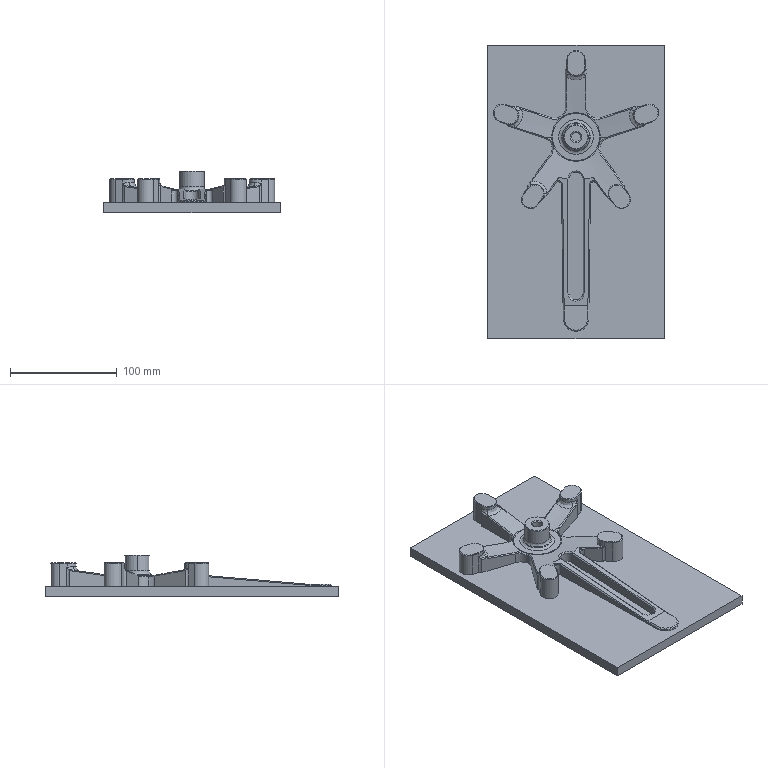Part | 1 solid | 152 faces | box 165 x 275 x 39 mm | volume 555031 mm3 | plane 57 | cylinder 37 | spline 33 | cone 22 | torus 3 | commonest cylinder face diameters 17 x14 6 x12 20 x5 13.2 x2 23 x2 8.6 x1